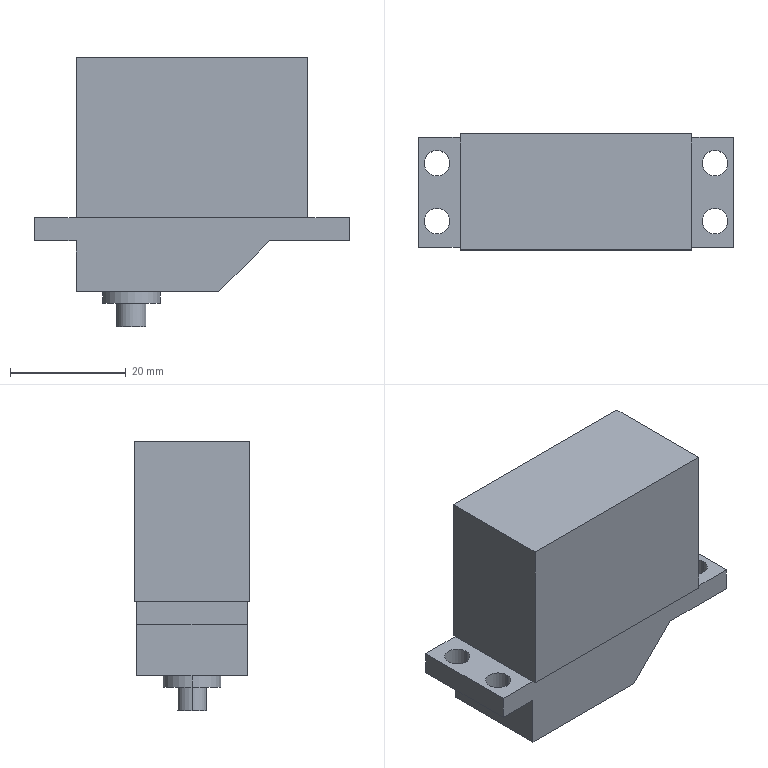Part | SolidWorks | features MirrorStock 1 | 1 solid | 32 faces | box 54.44 x 20 x 46.45 mm | volume 31100 mm3 | plane 20 | cylinder 12 | commonest cylinder face diameters 4.4 x8 5 x2 10 x2
STEP:
#1=CARTESIAN_POINT('',(-12.95,0.,-46.45));
#2=VERTEX_POINT('',#1);
#3=CARTESIAN_POINT('',(-7.95,0.,-46.45));
#4=VERTEX_POINT('',#3);
#5=CARTESIAN_POINT('',(-10.45,0.,-46.45));
#6=DIRECTION('',(0.,0.,1.));
#7=DIRECTION('',(1.,0.,0.));
#8=AXIS2_PLACEMENT_3D('',#5,#6,#7);
#9=CIRCLE('',#8,2.5);
#10=EDGE_CURVE('',#2,#4,#9,.T.);
#11=ORIENTED_EDGE('',*,*,#10,.T.);
#12=CARTESIAN_POINT('',(-7.95,0.,-42.45));
#13=VERTEX_POINT('',#12);
#14=CARTESIAN_POINT('',(-7.95,0.,-46.45));
#15=DIRECTION('',(0.,0.,1.));
#16=VECTOR('',#15,1000.);
#17=LINE('',#14,#16);
#18=EDGE_CURVE('',#4,#13,#17,.T.);
#19=ORIENTED_EDGE('',*,*,#18,.T.);
#20=CARTESIAN_POINT('',(-12.95,0.,-42.45));
#21=VERTEX_POINT('',#20);
#22=CARTESIAN_POINT('',(-10.45,0.,-42.45));
#23=DIRECTION('',(0.,0.,1.));
#24=DIRECTION('',(1.,0.,0.));
#25=AXIS2_PLACEMENT_3D('',#22,#23,#24);
#26=CIRCLE('',#25,2.5);
#27=EDGE_CURVE('',#21,#13,#26,.T.);
#28=ORIENTED_EDGE('',*,*,#27,.F.);
#29=CARTESIAN_POINT('',(-12.95,0.,-46.45));
#30=DIRECTION('',(0.,0.,1.));
#31=VECTOR('',#30,1000.);
#32=LINE('',#29,#31);
#33=EDGE_CURVE('',#2,#21,#32,.T.);
#34=ORIENTED_EDGE('',*,*,#33,.F.);
#35=EDGE_LOOP('',(#11,#19,#28,#34));
#36=FACE_OUTER_BOUND('',#35,.T.);
#37=CARTESIAN_POINT('',(-10.45,0.,-46.45));
#38=DIRECTION('',(0.,0.,1.));
#39=DIRECTION('',(-1.,0.,0.));
#40=AXIS2_PLACEMENT_3D('',#37,#38,#39);
#41=CYLINDRICAL_SURFACE('',#40,2.5);
#42=ADVANCED_FACE('',(#36),#41,.T.);
#43=CARTESIAN_POINT('',(-15.45,0.,-42.45));
#44=VERTEX_POINT('',#43);
#45=CARTESIAN_POINT('',(-5.45,0.,-42.45));
#46=VERTEX_POINT('',#45);
#47=CARTESIAN_POINT('',(-10.45,0.,-42.45));
#48=DIRECTION('',(0.,0.,1.));
#49=DIRECTION('',(1.,0.,0.));
#50=AXIS2_PLACEMENT_3D('',#47,#48,#49);
#51=CIRCLE('',#50,5.);
#52=EDGE_CURVE('',#44,#46,#51,.T.);
#53=ORIENTED_EDGE('',*,*,#52,.T.);
#54=CARTESIAN_POINT('',(-5.45,0.,-40.45));
#55=VERTEX_POINT('',#54);
#56=CARTESIAN_POINT('',(-5.45,0.,-42.45));
#57=DIRECTION('',(0.,0.,1.));
#58=VECTOR('',#57,1000.);
#59=LINE('',#56,#58);
#60=EDGE_CURVE('',#46,#55,#59,.T.);
#61=ORIENTED_EDGE('',*,*,#60,.T.);
#62=CARTESIAN_POINT('',(-15.45,0.,-40.45));
#63=VERTEX_POINT('',#62);
#64=CARTESIAN_POINT('',(-10.45,0.,-40.45));
#65=DIRECTION('',(0.,0.,1.));
#66=DIRECTION('',(1.,0.,0.));
#67=AXIS2_PLACEMENT_3D('',#64,#65,#66);
#68=CIRCLE('',#67,5.);
#69=EDGE_CURVE('',#63,#55,#68,.T.);
#70=ORIENTED_EDGE('',*,*,#69,.F.);
#71=CARTESIAN_POINT('',(-15.45,0.,-42.45));
#72=DIRECTION('',(0.,0.,1.));
#73=VECTOR('',#72,1000.);
#74=LINE('',#71,#73);
#75=EDGE_CURVE('',#44,#63,#74,.T.);
#76=ORIENTED_EDGE('',*,*,#75,.F.);
#77=EDGE_LOOP('',(#53,#61,#70,#76));
#78=FACE_OUTER_BOUND('',#77,.T.);
#79=CARTESIAN_POINT('',(-10.45,0.,-42.45));
#80=DIRECTION('',(0.,0.,1.));
#81=DIRECTION('',(-1.,0.,0.));
#82=AXIS2_PLACEMENT_3D('',#79,#80,#81);
#83=CYLINDRICAL_SURFACE('',#82,5.);
#84=ADVANCED_FACE('',(#78),#83,.T.);
#85=CARTESIAN_POINT('',(26.2,5.,-27.65));
#86=VERTEX_POINT('',#85);
#87=CARTESIAN_POINT('',(21.8,5.,-27.65));
#88=VERTEX_POINT('',#87);
#89=CARTESIAN_POINT('',(24.,5.,-27.65));
#90=DIRECTION('',(0.,0.,1.));
#91=DIRECTION('',(1.,0.,0.));
#92=AXIS2_PLACEMENT_3D('',#89,#90,#91);
#93=CIRCLE('',#92,2.2);
#94=EDGE_CURVE('',#86,#88,#93,.T.);
#95=ORIENTED_EDGE('',*,*,#94,.T.);
#96=CARTESIAN_POINT('',(21.8,5.,-31.65));
#97=VERTEX_POINT('',#96);
#98=CARTESIAN_POINT('',(21.8,5.,-27.65));
#99=DIRECTION('',(0.,0.,-1.));
#100=VECTOR('',#99,1000.);
#101=LINE('',#98,#100);
#102=EDGE_CURVE('',#88,#97,#101,.T.);
#103=ORIENTED_EDGE('',*,*,#102,.T.);
#104=CARTESIAN_POINT('',(26.2,5.,-31.65));
#105=VERTEX_POINT('',#104);
#106=CARTESIAN_POINT('',(24.,5.,-31.65));
#107=DIRECTION('',(0.,0.,1.));
#108=DIRECTION('',(1.,0.,0.));
#109=AXIS2_PLACEMENT_3D('',#106,#107,#108);
#110=CIRCLE('',#109,2.2);
#111=EDGE_CURVE('',#105,#97,#110,.T.);
#112=ORIENTED_EDGE('',*,*,#111,.F.);
#113=CARTESIAN_POINT('',(26.2,5.,-27.65));
#114=DIRECTION('',(0.,0.,-1.));
#115=VECTOR('',#114,1000.);
#116=LINE('',#113,#115);
#117=EDGE_CURVE('',#86,#105,#116,.T.);
#118=ORIENTED_EDGE('',*,*,#117,.F.);
#119=EDGE_LOOP('',(#95,#103,#112,#118));
#120=FACE_OUTER_BOUND('',#119,.T.);
#121=CARTESIAN_POINT('',(24.,5.,-27.65));
#122=DIRECTION('',(0.,0.,-1.));
#123=DIRECTION('',(1.,0.,0.));
#124=AXIS2_PLACEMENT_3D('',#121,#122,#123);
#125=CYLINDRICAL_SURFACE('',#124,2.2);
#126=ADVANCED_FACE('',(#120),#125,.F.);
#127=CARTESIAN_POINT('',(26.2,-5.,-27.65));
#128=VERTEX_POINT('',#127);
#129=CARTESIAN_POINT('',(21.8,-5.,-27.65));
#130=VERTEX_POINT('',#129);
#131=CARTESIAN_POINT('',(24.,-5.,-27.65));
#132=DIRECTION('',(0.,0.,1.));
#133=DIRECTION('',(1.,0.,0.));
#134=AXIS2_PLACEMENT_3D('',#131,#132,#133);
#135=CIRCLE('',#134,2.2);
#136=EDGE_CURVE('',#128,#130,#135,.T.);
#137=ORIENTED_EDGE('',*,*,#136,.T.);
#138=CARTESIAN_POINT('',(21.8,-5.,-31.65));
#139=VERTEX_POINT('',#138);
#140=CARTESIAN_POINT('',(21.8,-5.,-27.65));
#141=DIRECTION('',(0.,0.,-1.));
#142=VECTOR('',#141,1000.);
#143=LINE('',#140,#142);
#144=EDGE_CURVE('',#130,#139,#143,.T.);
#145=ORIENTED_EDGE('',*,*,#144,.T.);
#146=CARTESIAN_POINT('',(26.2,-5.,-31.65));
#147=VERTEX_POINT('',#146);
#148=CARTESIAN_POINT('',(24.,-5.,-31.65));
#149=DIRECTION('',(0.,0.,1.));
#150=DIRECTION('',(1.,0.,0.));
#151=AXIS2_PLACEMENT_3D('',#148,#149,#150);
#152=CIRCLE('',#151,2.2);
#153=EDGE_CURVE('',#147,#139,#152,.T.);
#154=ORIENTED_EDGE('',*,*,#153,.F.);
#155=CARTESIAN_POINT('',(26.2,-5.,-27.65));
#156=DIRECTION('',(0.,0.,-1.));
#157=VECTOR('',#156,1000.);
#158=LINE('',#155,#157);
#159=EDGE_CURVE('',#128,#147,#158,.T.);
#160=ORIENTED_EDGE('',*,*,#159,.F.);
#161=EDGE_LOOP('',(#137,#145,#154,#160));
#162=FACE_OUTER_BOUND('',#161,.T.);
#163=CARTESIAN_POINT('',(24.,-5.,-27.65));
#164=DIRECTION('',(0.,0.,-1.));
#165=DIRECTION('',(1.,0.,0.));
#166=AXIS2_PLACEMENT_3D('',#163,#164,#165);
#167=CYLINDRICAL_SURFACE('',#166,2.2);
#168=ADVANCED_FACE('',(#162),#167,.F.);
#169=CARTESIAN_POINT('',(-21.8,-5.,-27.65));
#170=VERTEX_POINT('',#169);
#171=CARTESIAN_POINT('',(-26.2,-5.,-27.65));
#172=VERTEX_POINT('',#171);
#173=CARTESIAN_POINT('',(-24.,-5.,-27.65));
#174=DIRECTION('',(0.,0.,1.));
#175=DIRECTION('',(1.,0.,0.));
#176=AXIS2_PLACEMENT_3D('',#173,#174,#175);
#177=CIRCLE('',#176,2.2);
#178=EDGE_CURVE('',#170,#172,#177,.T.);
#179=ORIENTED_EDGE('',*,*,#178,.T.);
#180=CARTESIAN_POINT('',(-26.2,-5.,-31.65));
#181=VERTEX_POINT('',#180);
#182=CARTESIAN_POINT('',(-26.2,-5.,-27.65));
#183=DIRECTION('',(0.,0.,-1.));
#184=VECTOR('',#183,1000.);
#185=LINE('',#182,#184);
#186=EDGE_CURVE('',#172,#181,#185,.T.);
#187=ORIENTED_EDGE('',*,*,#186,.T.);
#188=CARTESIAN_POINT('',(-21.8,-5.,-31.65));
#189=VERTEX_POINT('',#188);
#190=CARTESIAN_POINT('',(-24.,-5.,-31.65));
#191=DIRECTION('',(0.,0.,1.));
#192=DIRECTION('',(1.,0.,0.));
#193=AXIS2_PLACEMENT_3D('',#190,#191,#192);
#194=CIRCLE('',#193,2.2);
#195=EDGE_CURVE('',#189,#181,#194,.T.);
#196=ORIENTED_EDGE('',*,*,#195,.F.);
#197=CARTESIAN_POINT('',(-21.8,-5.,-27.65));
#198=DIRECTION('',(0.,0.,-1.));
#199=VECTOR('',#198,1000.);
#200=LINE('',#197,#199);
#201=EDGE_CURVE('',#170,#189,#200,.T.);
#202=ORIENTED_EDGE('',*,*,#201,.F.);
#203=EDGE_LOOP('',(#179,#187,#196,#202));
#204=FACE_OUTER_BOUND('',#203,.T.);
#205=CARTESIAN_POINT('',(-24.,-5.,-27.65));
#206=DIRECTION('',(0.,0.,-1.));
#207=DIRECTION('',(1.,0.,0.));
#208=AXIS2_PLACEMENT_3D('',#205,#206,#207);
#209=CYLINDRICAL_SURFACE('',#208,2.2);
#210=ADVANCED_FACE('',(#204),#209,.F.);
#211=CARTESIAN_POINT('',(-21.8,5.,-27.65));
#212=VERTEX_POINT('',#211);
#213=CARTESIAN_POINT('',(-26.2,5.,-27.65));
#214=VERTEX_POINT('',#213);
#215=CARTESIAN_POINT('',(-24.,5.,-27.65));
#216=DIRECTION('',(0.,0.,1.));
#217=DIRECTION('',(1.,0.,0.));
#218=AXIS2_PLACEMENT_3D('',#215,#216,#217);
#219=CIRCLE('',#218,2.2);
#220=EDGE_CURVE('',#212,#214,#219,.T.);
#221=ORIENTED_EDGE('',*,*,#220,.T.);
#222=CARTESIAN_POINT('',(-26.2,5.,-31.65));
#223=VERTEX_POINT('',#222);
#224=CARTESIAN_POINT('',(-26.2,5.,-27.65));
#225=DIRECTION('',(0.,0.,-1.));
#226=VECTOR('',#225,1000.);
#227=LINE('',#224,#226);
#228=EDGE_CURVE('',#214,#223,#227,.T.);
#229=ORIENTED_EDGE('',*,*,#228,.T.);
#230=CARTESIAN_POINT('',(-21.8,5.,-31.65));
#231=VERTEX_POINT('',#230);
#232=CARTESIAN_POINT('',(-24.,5.,-31.65));
#233=DIRECTION('',(0.,0.,1.));
#234=DIRECTION('',(1.,0.,0.));
#235=AXIS2_PLACEMENT_3D('',#232,#233,#234);
#236=CIRCLE('',#235,2.2);
#237=EDGE_CURVE('',#231,#223,#236,.T.);
#238=ORIENTED_EDGE('',*,*,#237,.F.);
#239=CARTESIAN_POINT('',(-21.8,5.,-27.65));
#240=DIRECTION('',(0.,0.,-1.));
#241=VECTOR('',#240,1000.);
#242=LINE('',#239,#241);
#243=EDGE_CURVE('',#212,#231,#242,.T.);
#244=ORIENTED_EDGE('',*,*,#243,.F.);
#245=EDGE_LOOP('',(#221,#229,#238,#244));
#246=FACE_OUTER_BOUND('',#245,.T.);
#247=CARTESIAN_POINT('',(-24.,5.,-27.65));
#248=DIRECTION('',(0.,0.,-1.));
#249=DIRECTION('',(1.,0.,0.));
#250=AXIS2_PLACEMENT_3D('',#247,#248,#249);
#251=CYLINDRICAL_SURFACE('',#250,2.2);
#252=ADVANCED_FACE('',(#246),#251,.F.);
#253=CARTESIAN_POINT('',(-20.,9.5,-31.65));
#254=VERTEX_POINT('',#253);
#255=CARTESIAN_POINT('',(-20.,-9.5,-31.65));
#256=VERTEX_POINT('',#255);
#257=CARTESIAN_POINT('',(-20.,-9.5,-31.65));
#258=DIRECTION('',(0.,-1.,0.));
#259=VECTOR('',#258,1000.);
#260=LINE('',#257,#259);
#261=EDGE_CURVE('',#254,#256,#260,.T.);
#262=ORIENTED_EDGE('',*,*,#261,.T.);
#263=CARTESIAN_POINT('',(-27.22,-9.5,-31.65));
#264=VERTEX_POINT('',#263);
#265=CARTESIAN_POINT('',(27.22,-9.5,-31.65));
#266=DIRECTION('',(1.,0.,0.));
#267=VECTOR('',#266,1000.);
#268=LINE('',#265,#267);
#269=EDGE_CURVE('',#264,#256,#268,.T.);
#270=ORIENTED_EDGE('',*,*,#269,.F.);
#271=CARTESIAN_POINT('',(-27.22,9.5,-31.65));
#272=VERTEX_POINT('',#271);
#273=CARTESIAN_POINT('',(-27.22,-9.5,-31.65));
#274=DIRECTION('',(0.,-1.,0.));
#275=VECTOR('',#274,1000.);
#276=LINE('',#273,#275);
#277=EDGE_CURVE('',#272,#264,#276,.T.);
#278=ORIENTED_EDGE('',*,*,#277,.F.);
#279=CARTESIAN_POINT('',(27.22,9.5,-31.65));
#280=DIRECTION('',(-1.,0.,0.));
#281=VECTOR('',#280,1000.);
#282=LINE('',#279,#281);
#283=EDGE_CURVE('',#254,#272,#282,.T.);
#284=ORIENTED_EDGE('',*,*,#283,.F.);
#285=EDGE_LOOP('',(#262,#270,#278,#284));
#286=FACE_OUTER_BOUND('',#285,.T.);
#287=ORIENTED_EDGE('',*,*,#237,.T.);
#288=CARTESIAN_POINT('',(-24.,5.,-31.65));
#289=DIRECTION('',(0.,0.,1.));
#290=DIRECTION('',(1.,0.,0.));
#291=AXIS2_PLACEMENT_3D('',#288,#289,#290);
#292=CIRCLE('',#291,2.2);
#293=EDGE_CURVE('',#223,#231,#292,.T.);
#294=ORIENTED_EDGE('',*,*,#293,.T.);
#295=EDGE_LOOP('',(#287,#294));
#296=FACE_BOUND('',#295,.T.);
#297=ORIENTED_EDGE('',*,*,#195,.T.);
#298=CARTESIAN_POINT('',(-24.,-5.,-31.65));
#299=DIRECTION('',(0.,0.,1.));
#300=DIRECTION('',(1.,0.,0.));
#301=AXIS2_PLACEMENT_3D('',#298,#299,#300);
#302=CIRCLE('',#301,2.2);
#303=EDGE_CURVE('',#181,#189,#302,.T.);
#304=ORIENTED_EDGE('',*,*,#303,.T.);
#305=EDGE_LOOP('',(#297,#304));
#306=FACE_BOUND('',#305,.T.);
#307=CARTESIAN_POINT('',(0.,0.,-31.65));
#308=DIRECTION('',(0.,0.,-1.));
#309=DIRECTION('',(1.,0.,0.));
#310=AXIS2_PLACEMENT_3D('',#307,#308,#309);
#311=PLANE('',#310);
#312=ADVANCED_FACE('',(#286,#296,#306),#311,.T.);
#313=CARTESIAN_POINT('',(20.,9.5,-27.65));
#314=VERTEX_POINT('',#313);
#315=CARTESIAN_POINT('',(-20.,9.5,-27.65));
#316=VERTEX_POINT('',#315);
#317=CARTESIAN_POINT('',(27.22,9.5,-27.65));
#318=DIRECTION('',(-1.,0.,0.));
#319=VECTOR('',#318,1000.);
#320=LINE('',#317,#319);
#321=EDGE_CURVE('',#314,#316,#320,.T.);
#322=ORIENTED_EDGE('',*,*,#321,.T.);
#323=CARTESIAN_POINT('',(-20.,10.,-27.65));
#324=VERTEX_POINT('',#323);
#325=CARTESIAN_POINT('',(-20.,-10.,-27.65));
#326=DIRECTION('',(0.,-1.,0.));
#327=VECTOR('',#326,1000.);
#328=LINE('',#325,#327);
#329=EDGE_CURVE('',#324,#316,#328,.T.);
#330=ORIENTED_EDGE('',*,*,#329,.F.);
#331=CARTESIAN_POINT('',(20.,10.,-27.65));
#332=VERTEX_POINT('',#331);
#333=CARTESIAN_POINT('',(20.,10.,-27.65));
#334=DIRECTION('',(-1.,0.,0.));
#335=VECTOR('',#334,1000.);
#336=LINE('',#333,#335);
#337=EDGE_CURVE('',#332,#324,#336,.T.);
#338=ORIENTED_EDGE('',*,*,#337,.F.);
#339=CARTESIAN_POINT('',(20.,-10.,-27.65));
#340=DIRECTION('',(0.,1.,0.));
#341=VECTOR('',#340,1000.);
#342=LINE('',#339,#341);
#343=EDGE_CURVE('',#314,#332,#342,.T.);
#344=ORIENTED_EDGE('',*,*,#343,.F.);
#345=EDGE_LOOP('',(#322,#330,#338,#344));
#346=FACE_OUTER_BOUND('',#345,.T.);
#347=CARTESIAN_POINT('',(0.,0.,-27.65));
#348=DIRECTION('',(0.,0.,-1.));
#349=DIRECTION('',(1.,0.,0.));
#350=AXIS2_PLACEMENT_3D('',#347,#348,#349);
#351=PLANE('',#350);
#352=ADVANCED_FACE('',(#346),#351,.T.);
#353=CARTESIAN_POINT('',(-20.,10.,0.));
#354=VERTEX_POINT('',#353);
#355=CARTESIAN_POINT('',(-20.,-10.,0.));
#356=VERTEX_POINT('',#355);
#357=CARTESIAN_POINT('',(-20.,-10.,0.));
#358=DIRECTION('',(0.,-1.,0.));
#359=VECTOR('',#358,1000.);
#360=LINE('',#357,#359);
#361=EDGE_CURVE('',#354,#356,#360,.T.);
#362=ORIENTED_EDGE('',*,*,#361,.F.);
#363=CARTESIAN_POINT('',(-20.,10.,-27.65));
#364=DIRECTION('',(0.,0.,1.));
#365=VECTOR('',#364,1000.);
#366=LINE('',#363,#365);
#367=EDGE_CURVE('',#324,#354,#366,.T.);
#368=ORIENTED_EDGE('',*,*,#367,.F.);
#369=ORIENTED_EDGE('',*,*,#329,.T.);
#370=CARTESIAN_POINT('',(-20.,-9.5,-27.65));
#371=VERTEX_POINT('',#370);
#372=CARTESIAN_POINT('',(-20.,-10.,-27.65));
#373=DIRECTION('',(0.,-1.,0.));
#374=VECTOR('',#373,1000.);
#375=LINE('',#372,#374);
#376=EDGE_CURVE('',#316,#371,#375,.T.);
#377=ORIENTED_EDGE('',*,*,#376,.T.);
#378=CARTESIAN_POINT('',(-20.,-10.,-27.65));
#379=VERTEX_POINT('',#378);
#380=CARTESIAN_POINT('',(-20.,-10.,-27.65));
#381=DIRECTION('',(0.,-1.,0.));
#382=VECTOR('',#381,1000.);
#383=LINE('',#380,#382);
#384=EDGE_CURVE('',#371,#379,#383,.T.);
#385=ORIENTED_EDGE('',*,*,#384,.T.);
#386=CARTESIAN_POINT('',(-20.,-10.,-27.65));
#387=DIRECTION('',(0.,0.,1.));
#388=VECTOR('',#387,1000.);
#389=LINE('',#386,#388);
#390=EDGE_CURVE('',#379,#356,#389,.T.);
#391=ORIENTED_EDGE('',*,*,#390,.T.);
#392=EDGE_LOOP('',(#362,#368,#369,#377,#385,#391));
#393=FACE_OUTER_BOUND('',#392,.T.);
#394=CARTESIAN_POINT('',(-20.,-10.,-27.65));
#395=DIRECTION('',(1.,0.,0.));
#396=DIRECTION('',(0.,0.,1.));
#397=AXIS2_PLACEMENT_3D('',#394,#395,#396);
#398=PLANE('',#397);
#399=ADVANCED_FACE('',(#393),#398,.F.);
#400=CARTESIAN_POINT('',(20.,-10.,0.));
#401=VERTEX_POINT('',#400);
#402=CARTESIAN_POINT('',(20.,-10.,0.));
#403=DIRECTION('',(1.,0.,0.));
#404=VECTOR('',#403,1000.);
#405=LINE('',#402,#404);
#406=EDGE_CURVE('',#356,#401,#405,.T.);
#407=ORIENTED_EDGE('',*,*,#406,.F.);
#408=ORIENTED_EDGE('',*,*,#390,.F.);
#409=CARTESIAN_POINT('',(20.,-10.,-27.65));
#410=VERTEX_POINT('',#409);
#411=CARTESIAN_POINT('',(20.,-10.,-27.65));
#412=DIRECTION('',(1.,0.,0.));
#413=VECTOR('',#412,1000.);
#414=LINE('',#411,#413);
#415=EDGE_CURVE('',#379,#410,#414,.T.);
#416=ORIENTED_EDGE('',*,*,#415,.T.);
#417=CARTESIAN_POINT('',(20.,-10.,-27.65));
#418=DIRECTION('',(0.,0.,1.));
#419=VECTOR('',#418,1000.);
#420=LINE('',#417,#419);
#421=EDGE_CURVE('',#410,#401,#420,.T.);
#422=ORIENTED_EDGE('',*,*,#421,.T.);
#423=EDGE_LOOP('',(#407,#408,#416,#422));
#424=FACE_OUTER_BOUND('',#423,.T.);
#425=CARTESIAN_POINT('',(20.,-10.,-27.65));
#426=DIRECTION('',(0.,1.,0.));
#427=DIRECTION('',(-1.,0.,0.));
#428=AXIS2_PLACEMENT_3D('',#425,#426,#427);
#429=PLANE('',#428);
#430=ADVANCED_FACE('',(#424),#429,.F.);
#431=CARTESIAN_POINT('',(20.,10.,0.));
#432=VERTEX_POINT('',#431);
#433=CARTESIAN_POINT('',(20.,-10.,0.));
#434=DIRECTION('',(0.,1.,0.));
#435=VECTOR('',#434,1000.);
#436=LINE('',#433,#435);
#437=EDGE_CURVE('',#401,#432,#436,.T.);
#438=ORIENTED_EDGE('',*,*,#437,.F.);
#439=ORIENTED_EDGE('',*,*,#421,.F.);
#440=CARTESIAN_POINT('',(20.,-9.5,-27.65));
#441=VERTEX_POINT('',#440);
#442=CARTESIAN_POINT('',(20.,-10.,-27.65));
#443=DIRECTION('',(0.,1.,0.));
#444=VECTOR('',#443,1000.);
#445=LINE('',#442,#444);
#446=EDGE_CURVE('',#410,#441,#445,.T.);
#447=ORIENTED_EDGE('',*,*,#446,.T.);
#448=CARTESIAN_POINT('',(20.,-10.,-27.65));
#449=DIRECTION('',(0.,1.,0.));
#450=VECTOR('',#449,1000.);
#451=LINE('',#448,#450);
#452=EDGE_CURVE('',#441,#314,#451,.T.);
#453=ORIENTED_EDGE('',*,*,#452,.T.);
#454=ORIENTED_EDGE('',*,*,#343,.T.);
#455=CARTESIAN_POINT('',(20.,10.,-27.65));
#456=DIRECTION('',(0.,0.,1.));
#457=VECTOR('',#456,1000.);
#458=LINE('',#455,#457);
#459=EDGE_CURVE('',#332,#432,#458,.T.);
#460=ORIENTED_EDGE('',*,*,#459,.T.);
#461=EDGE_LOOP('',(#438,#439,#447,#453,#454,#460));
#462=FACE_OUTER_BOUND('',#461,.T.);
#463=CARTESIAN_POINT('',(20.,-10.,-27.65));
#464=DIRECTION('',(-1.,0.,0.));
#465=DIRECTION('',(0.,0.,-1.));
#466=AXIS2_PLACEMENT_3D('',#463,#464,#465);
#467=PLANE('',#466);
#468=ADVANCED_FACE('',(#462),#467,.F.);
#469=CARTESIAN_POINT('',(20.,10.,0.));
#470=DIRECTION('',(-1.,0.,0.));
#471=VECTOR('',#470,1000.);
#472=LINE('',#469,#471);
#473=EDGE_CURVE('',#432,#354,#472,.T.);
#474=ORIENTED_EDGE('',*,*,#473,.F.);
#475=ORIENTED_EDGE('',*,*,#459,.F.);
#476=ORIENTED_EDGE('',*,*,#337,.T.);
#477=ORIENTED_EDGE('',*,*,#367,.T.);
#478=EDGE_LOOP('',(#474,#475,#476,#477));
#479=FACE_OUTER_BOUND('',#478,.T.);
#480=CARTESIAN_POINT('',(20.,10.,-27.65));
#481=DIRECTION('',(0.,-1.,0.));
#482=DIRECTION('',(1.,0.,0.));
#483=AXIS2_PLACEMENT_3D('',#480,#481,#482);
#484=PLANE('',#483);
#485=ADVANCED_FACE('',(#479),#484,.F.);
#486=CARTESIAN_POINT('',(27.22,-9.5,-27.65));
#487=DIRECTION('',(1.,0.,0.));
#488=VECTOR('',#487,1000.);
#489=LINE('',#486,#488);
#490=EDGE_CURVE('',#371,#441,#489,.T.);
#491=ORIENTED_EDGE('',*,*,#490,.T.);
#492=ORIENTED_EDGE('',*,*,#446,.F.);
#493=ORIENTED_EDGE('',*,*,#415,.F.);
#494=ORIENTED_EDGE('',*,*,#384,.F.);
#495=EDGE_LOOP('',(#491,#492,#493,#494));
#496=FACE_OUTER_BOUND('',#495,.T.);
#497=CARTESIAN_POINT('',(0.,0.,-27.65));
#498=DIRECTION('',(0.,0.,-1.));
#499=DIRECTION('',(1.,0.,0.));
#500=AXIS2_PLACEMENT_3D('',#497,#498,#499);
#501=PLANE('',#500);
#502=ADVANCED_FACE('',(#496),#501,.T.);
#503=ORIENTED_EDGE('',*,*,#361,.T.);
#504=ORIENTED_EDGE('',*,*,#406,.T.);
#505=ORIENTED_EDGE('',*,*,#437,.T.);
#506=ORIENTED_EDGE('',*,*,#473,.T.);
#507=EDGE_LOOP('',(#503,#504,#505,#506));
#508=FACE_OUTER_BOUND('',#507,.T.);
#509=CARTESIAN_POINT('',(0.,0.,0.));
#510=DIRECTION('',(0.,0.,-1.));
#511=DIRECTION('',(1.,0.,0.));
#512=AXIS2_PLACEMENT_3D('',#509,#510,#511);
#513=PLANE('',#512);
#514=ADVANCED_FACE('',(#508),#513,.F.);
#515=ORIENTED_EDGE('',*,*,#178,.F.);
#516=CARTESIAN_POINT('',(-24.,-5.,-27.65));
#517=DIRECTION('',(0.,0.,1.));
#518=DIRECTION('',(1.,0.,0.));
#519=AXIS2_PLACEMENT_3D('',#516,#517,#518);
#520=CIRCLE('',#519,2.2);
#521=EDGE_CURVE('',#172,#170,#520,.T.);
#522=ORIENTED_EDGE('',*,*,#521,.F.);
#523=EDGE_LOOP('',(#515,#522));
#524=FACE_BOUND('',#523,.T.);
#525=ORIENTED_EDGE('',*,*,#220,.F.);
#526=CARTESIAN_POINT('',(-24.,5.,-27.65));
#527=DIRECTION('',(0.,0.,1.));
#528=DIRECTION('',(1.,0.,0.));
#529=AXIS2_PLACEMENT_3D('',#526,#527,#528);
#530=CIRCLE('',#529,2.2);
#531=EDGE_CURVE('',#214,#212,#530,.T.);
#532=ORIENTED_EDGE('',*,*,#531,.F.);
#533=EDGE_LOOP('',(#525,#532));
#534=FACE_BOUND('',#533,.T.);
#535=CARTESIAN_POINT('',(-27.22,9.5,-27.65));
#536=VERTEX_POINT('',#535);
#537=CARTESIAN_POINT('',(27.22,9.5,-27.65));
#538=DIRECTION('',(-1.,0.,0.));
#539=VECTOR('',#538,1000.);
#540=LINE('',#537,#539);
#541=EDGE_CURVE('',#316,#536,#540,.T.);
#542=ORIENTED_EDGE('',*,*,#541,.T.);
#543=CARTESIAN_POINT('',(-27.22,-9.5,-27.65));
#544=VERTEX_POINT('',#543);
#545=CARTESIAN_POINT('',(-27.22,-9.5,-27.65));
#546=DIRECTION('',(0.,-1.,0.));
#547=VECTOR('',#546,1000.);
#548=LINE('',#545,#547);
#549=EDGE_CURVE('',#536,#544,#548,.T.);
#550=ORIENTED_EDGE('',*,*,#549,.T.);
#551=CARTESIAN_POINT('',(27.22,-9.5,-27.65));
#552=DIRECTION('',(1.,0.,0.));
#553=VECTOR('',#552,1000.);
#554=LINE('',#551,#553);
#555=EDGE_CURVE('',#544,#371,#554,.T.);
#556=ORIENTED_EDGE('',*,*,#555,.T.);
#557=ORIENTED_EDGE('',*,*,#376,.F.);
#558=EDGE_LOOP('',(#542,#550,#556,#557));
#559=FACE_OUTER_BOUND('',#558,.T.);
#560=CARTESIAN_POINT('',(0.,0.,-27.65));
#561=DIRECTION('',(0.,0.,-1.));
#562=DIRECTION('',(1.,0.,0.));
#563=AXIS2_PLACEMENT_3D('',#560,#561,#562);
#564=PLANE('',#563);
#565=ADVANCED_FACE('',(#524,#534,#559),#564,.F.);
#566=ORIENTED_EDGE('',*,*,#94,.F.);
#567=CARTESIAN_POINT('',(24.,5.,-27.65));
#568=DIRECTION('',(0.,0.,1.));
#569=DIRECTION('',(1.,0.,0.));
#570=AXIS2_PLACEMENT_3D('',#567,#568,#569);
#571=CIRCLE('',#570,2.2);
#572=EDGE_CURVE('',#88,#86,#571,.T.);
#573=ORIENTED_EDGE('',*,*,#572,.F.);
#574=EDGE_LOOP('',(#566,#573));
#575=FACE_BOUND('',#574,.T.);
#576=ORIENTED_EDGE('',*,*,#136,.F.);
#577=CARTESIAN_POINT('',(24.,-5.,-27.65));
#578=DIRECTION('',(0.,0.,1.));
#579=DIRECTION('',(1.,0.,0.));
#580=AXIS2_PLACEMENT_3D('',#577,#578,#579);
#581=CIRCLE('',#580,2.2);
#582=EDGE_CURVE('',#130,#128,#581,.T.);
#583=ORIENTED_EDGE('',*,*,#582,.F.);
#584=EDGE_LOOP('',(#576,#583));
#585=FACE_BOUND('',#584,.T.);
#586=CARTESIAN_POINT('',(27.22,-9.5,-27.65));
#587=VERTEX_POINT('',#586);
#588=CARTESIAN_POINT('',(27.22,-9.5,-27.65));
#589=DIRECTION('',(1.,0.,0.));
#590=VECTOR('',#589,1000.);
#591=LINE('',#588,#590);
#592=EDGE_CURVE('',#441,#587,#591,.T.);
#593=ORIENTED_EDGE('',*,*,#592,.T.);
#594=CARTESIAN_POINT('',(27.22,9.5,-27.65));
#595=VERTEX_POINT('',#594);
#596=CARTESIAN_POINT('',(27.22,-9.5,-27.65));
#597=DIRECTION('',(0.,1.,0.));
#598=VECTOR('',#597,1000.);
#599=LINE('',#596,#598);
#600=EDGE_CURVE('',#587,#595,#599,.T.);
#601=ORIENTED_EDGE('',*,*,#600,.T.);
#602=CARTESIAN_POINT('',(27.22,9.5,-27.65));
#603=DIRECTION('',(-1.,0.,0.));
#604=VECTOR('',#603,1000.);
#605=LINE('',#602,#604);
#606=EDGE_CURVE('',#595,#314,#605,.T.);
#607=ORIENTED_EDGE('',*,*,#606,.T.);
#608=ORIENTED_EDGE('',*,*,#452,.F.);
#609=EDGE_LOOP('',(#593,#601,#607,#608));
#610=FACE_OUTER_BOUND('',#609,.T.);
#611=CARTESIAN_POINT('',(0.,0.,-27.65));
#612=DIRECTION('',(0.,0.,-1.));
#613=DIRECTION('',(1.,0.,0.));
#614=AXIS2_PLACEMENT_3D('',#611,#612,#613);
#615=PLANE('',#614);
#616=ADVANCED_FACE('',(#575,#585,#610),#615,.F.);
#617=ORIENTED_EDGE('',*,*,#549,.F.);
#618=CARTESIAN_POINT('',(-27.22,9.5,-31.65));
#619=DIRECTION('',(0.,0.,1.));
#620=VECTOR('',#619,1000.);
#621=LINE('',#618,#620);
#622=EDGE_CURVE('',#272,#536,#621,.T.);
#623=ORIENTED_EDGE('',*,*,#622,.F.);
#624=ORIENTED_EDGE('',*,*,#277,.T.);
#625=CARTESIAN_POINT('',(-27.22,-9.5,-31.65));
#626=DIRECTION('',(0.,0.,1.));
#627=VECTOR('',#626,1000.);
#628=LINE('',#625,#627);
#629=EDGE_CURVE('',#264,#544,#628,.T.);
#630=ORIENTED_EDGE('',*,*,#629,.T.);
#631=EDGE_LOOP('',(#617,#623,#624,#630));
#632=FACE_OUTER_BOUND('',#631,.T.);
#633=CARTESIAN_POINT('',(-27.22,-9.5,-31.65));
#634=DIRECTION('',(1.,0.,0.));
#635=DIRECTION('',(0.,0.,1.));
#636=AXIS2_PLACEMENT_3D('',#633,#634,#635);
#637=PLANE('',#636);
#638=ADVANCED_FACE('',(#632),#637,.F.);
#639=CARTESIAN_POINT('',(13.407,-9.5,-31.65));
#640=VERTEX_POINT('',#639);
#641=CARTESIAN_POINT('',(27.22,-9.5,-31.65));
#642=VERTEX_POINT('',#641);
#643=CARTESIAN_POINT('',(27.22,-9.5,-31.65));
#644=DIRECTION('',(1.,0.,0.));
#645=VECTOR('',#644,1000.);
#646=LINE('',#643,#645);
#647=EDGE_CURVE('',#640,#642,#646,.T.);
#648=ORIENTED_EDGE('',*,*,#647,.T.);
#649=CARTESIAN_POINT('',(27.22,-9.5,-31.65));
#650=DIRECTION('',(0.,0.,1.));
#651=VECTOR('',#650,1000.);
#652=LINE('',#649,#651);
#653=EDGE_CURVE('',#642,#587,#652,.T.);
#654=ORIENTED_EDGE('',*,*,#653,.T.);
#655=ORIENTED_EDGE('',*,*,#592,.F.);
#656=ORIENTED_EDGE('',*,*,#490,.F.);
#657=ORIENTED_EDGE('',*,*,#555,.F.);
#658=ORIENTED_EDGE('',*,*,#629,.F.);
#659=ORIENTED_EDGE('',*,*,#269,.T.);
#660=CARTESIAN_POINT('',(-20.,-9.5,-40.45));
#661=VERTEX_POINT('',#660);
#662=CARTESIAN_POINT('',(-20.,-9.5,-120.38));
#663=DIRECTION('',(0.,0.,1.));
#664=VECTOR('',#663,1000.);
#665=LINE('',#662,#664);
#666=EDGE_CURVE('',#661,#256,#665,.T.);
#667=ORIENTED_EDGE('',*,*,#666,.F.);
#668=CARTESIAN_POINT('',(4.607,-9.5,-40.45));
#669=VERTEX_POINT('',#668);
#670=CARTESIAN_POINT('',(14.607,-9.5,-40.45));
#671=DIRECTION('',(1.,0.,0.));
#672=VECTOR('',#671,1000.);
#673=LINE('',#670,#672);
#674=EDGE_CURVE('',#661,#669,#673,.T.);
#675=ORIENTED_EDGE('',*,*,#674,.T.);
#676=CARTESIAN_POINT('',(4.607,-9.5,-40.45));
#677=DIRECTION('',(-0.7071,0.,-0.7071));
#678=VECTOR('',#677,1000.);
#679=LINE('',#676,#678);
#680=EDGE_CURVE('',#640,#669,#679,.T.);
#681=ORIENTED_EDGE('',*,*,#680,.F.);
#682=EDGE_LOOP('',(#648,#654,#655,#656,#657,#658,#659,#667,#675,#681));
#683=FACE_OUTER_BOUND('',#682,.T.);
#684=CARTESIAN_POINT('',(27.22,-9.5,-31.65));
#685=DIRECTION('',(0.,1.,0.));
#686=DIRECTION('',(-1.,0.,0.));
#687=AXIS2_PLACEMENT_3D('',#684,#685,#686);
#688=PLANE('',#687);
#689=ADVANCED_FACE('',(#683),#688,.F.);
#690=ORIENTED_EDGE('',*,*,#600,.F.);
#691=ORIENTED_EDGE('',*,*,#653,.F.);
#692=CARTESIAN_POINT('',(27.22,9.5,-31.65));
#693=VERTEX_POINT('',#692);
#694=CARTESIAN_POINT('',(27.22,-9.5,-31.65));
#695=DIRECTION('',(0.,1.,0.));
#696=VECTOR('',#695,1000.);
#697=LINE('',#694,#696);
#698=EDGE_CURVE('',#642,#693,#697,.T.);
#699=ORIENTED_EDGE('',*,*,#698,.T.);
#700=CARTESIAN_POINT('',(27.22,9.5,-31.65));
#701=DIRECTION('',(0.,0.,1.));
#702=VECTOR('',#701,1000.);
#703=LINE('',#700,#702);
#704=EDGE_CURVE('',#693,#595,#703,.T.);
#705=ORIENTED_EDGE('',*,*,#704,.T.);
#706=EDGE_LOOP('',(#690,#691,#699,#705));
#707=FACE_OUTER_BOUND('',#706,.T.);
#708=CARTESIAN_POINT('',(27.22,-9.5,-31.65));
#709=DIRECTION('',(-1.,0.,0.));
#710=DIRECTION('',(0.,0.,-1.));
#711=AXIS2_PLACEMENT_3D('',#708,#709,#710);
#712=PLANE('',#711);
#713=ADVANCED_FACE('',(#707),#712,.F.);
#714=CARTESIAN_POINT('',(4.607,9.5,-40.45));
#715=VERTEX_POINT('',#714);
#716=CARTESIAN_POINT('',(13.407,9.5,-31.65));
#717=VERTEX_POINT('',#716);
#718=CARTESIAN_POINT('',(4.607,9.5,-40.45));
#719=DIRECTION('',(0.7071,0.,0.7071));
#720=VECTOR('',#719,1000.);
#721=LINE('',#718,#720);
#722=EDGE_CURVE('',#715,#717,#721,.T.);
#723=ORIENTED_EDGE('',*,*,#722,.F.);
#724=CARTESIAN_POINT('',(-20.,9.5,-40.45));
#725=VERTEX_POINT('',#724);
#726=CARTESIAN_POINT('',(14.607,9.5,-40.45));
#727=DIRECTION('',(-1.,0.,0.));
#728=VECTOR('',#727,1000.);
#729=LINE('',#726,#728);
#730=EDGE_CURVE('',#715,#725,#729,.T.);
#731=ORIENTED_EDGE('',*,*,#730,.T.);
#732=CARTESIAN_POINT('',(-20.,9.5,-120.38));
#733=DIRECTION('',(0.,0.,1.));
#734=VECTOR('',#733,1000.);
#735=LINE('',#732,#734);
#736=EDGE_CURVE('',#725,#254,#735,.T.);
#737=ORIENTED_EDGE('',*,*,#736,.T.);
#738=ORIENTED_EDGE('',*,*,#283,.T.);
#739=ORIENTED_EDGE('',*,*,#622,.T.);
#740=ORIENTED_EDGE('',*,*,#541,.F.);
#741=ORIENTED_EDGE('',*,*,#321,.F.);
#742=ORIENTED_EDGE('',*,*,#606,.F.);
#743=ORIENTED_EDGE('',*,*,#704,.F.);
#744=CARTESIAN_POINT('',(27.22,9.5,-31.65));
#745=DIRECTION('',(-1.,0.,0.));
#746=VECTOR('',#745,1000.);
#747=LINE('',#744,#746);
#748=EDGE_CURVE('',#693,#717,#747,.T.);
#749=ORIENTED_EDGE('',*,*,#748,.T.);
#750=EDGE_LOOP('',(#723,#731,#737,#738,#739,#740,#741,#742,#743,#749));
#751=FACE_OUTER_BOUND('',#750,.T.);
#752=CARTESIAN_POINT('',(27.22,9.5,-31.65));
#753=DIRECTION('',(0.,-1.,0.));
#754=DIRECTION('',(1.,0.,0.));
#755=AXIS2_PLACEMENT_3D('',#752,#753,#754);
#756=PLANE('',#755);
#757=ADVANCED_FACE('',(#751),#756,.F.);
#758=ORIENTED_EDGE('',*,*,#748,.F.);
#759=ORIENTED_EDGE('',*,*,#698,.F.);
#760=ORIENTED_EDGE('',*,*,#647,.F.);
#761=CARTESIAN_POINT('',(13.407,0.,-31.65));
#762=DIRECTION('',(0.,-1.,0.));
#763=VECTOR('',#762,1000.);
#764=LINE('',#761,#763);
#765=EDGE_CURVE('',#717,#640,#764,.T.);
#766=ORIENTED_EDGE('',*,*,#765,.F.);
#767=EDGE_LOOP('',(#758,#759,#760,#766));
#768=FACE_OUTER_BOUND('',#767,.T.);
#769=ORIENTED_EDGE('',*,*,#111,.T.);
#770=CARTESIAN_POINT('',(24.,5.,-31.65));
#771=DIRECTION('',(0.,0.,1.));
#772=DIRECTION('',(1.,0.,0.));
#773=AXIS2_PLACEMENT_3D('',#770,#771,#772);
#774=CIRCLE('',#773,2.2);
#775=EDGE_CURVE('',#97,#105,#774,.T.);
#776=ORIENTED_EDGE('',*,*,#775,.T.);
#777=EDGE_LOOP('',(#769,#776));
#778=FACE_BOUND('',#777,.T.);
#779=ORIENTED_EDGE('',*,*,#153,.T.);
#780=CARTESIAN_POINT('',(24.,-5.,-31.65));
#781=DIRECTION('',(0.,0.,1.));
#782=DIRECTION('',(1.,0.,0.));
#783=AXIS2_PLACEMENT_3D('',#780,#781,#782);
#784=CIRCLE('',#783,2.2);
#785=EDGE_CURVE('',#139,#147,#784,.T.);
#786=ORIENTED_EDGE('',*,*,#785,.T.);
#787=EDGE_LOOP('',(#779,#786));
#788=FACE_BOUND('',#787,.T.);
#789=CARTESIAN_POINT('',(0.,0.,-31.65));
#790=DIRECTION('',(0.,0.,-1.));
#791=DIRECTION('',(1.,0.,0.));
#792=AXIS2_PLACEMENT_3D('',#789,#790,#791);
#793=PLANE('',#792);
#794=ADVANCED_FACE('',(#768,#778,#788),#793,.T.);
#795=ORIENTED_EDGE('',*,*,#228,.F.);
#796=ORIENTED_EDGE('',*,*,#531,.T.);
#797=ORIENTED_EDGE('',*,*,#243,.T.);
#798=ORIENTED_EDGE('',*,*,#293,.F.);
#799=EDGE_LOOP('',(#795,#796,#797,#798));
#800=FACE_OUTER_BOUND('',#799,.T.);
#801=CARTESIAN_POINT('',(-24.,5.,-27.65));
#802=DIRECTION('',(0.,0.,-1.));
#803=DIRECTION('',(1.,0.,0.));
#804=AXIS2_PLACEMENT_3D('',#801,#802,#803);
#805=CYLINDRICAL_SURFACE('',#804,2.2);
#806=ADVANCED_FACE('',(#800),#805,.F.);
#807=ORIENTED_EDGE('',*,*,#186,.F.);
#808=ORIENTED_EDGE('',*,*,#521,.T.);
#809=ORIENTED_EDGE('',*,*,#201,.T.);
#810=ORIENTED_EDGE('',*,*,#303,.F.);
#811=EDGE_LOOP('',(#807,#808,#809,#810));
#812=FACE_OUTER_BOUND('',#811,.T.);
#813=CARTESIAN_POINT('',(-24.,-5.,-27.65));
#814=DIRECTION('',(0.,0.,-1.));
#815=DIRECTION('',(1.,0.,0.));
#816=AXIS2_PLACEMENT_3D('',#813,#814,#815);
#817=CYLINDRICAL_SURFACE('',#816,2.2);
#818=ADVANCED_FACE('',(#812),#817,.F.);
#819=ORIENTED_EDGE('',*,*,#144,.F.);
#820=ORIENTED_EDGE('',*,*,#582,.T.);
#821=ORIENTED_EDGE('',*,*,#159,.T.);
#822=ORIENTED_EDGE('',*,*,#785,.F.);
#823=EDGE_LOOP('',(#819,#820,#821,#822));
#824=FACE_OUTER_BOUND('',#823,.T.);
#825=CARTESIAN_POINT('',(24.,-5.,-27.65));
#826=DIRECTION('',(0.,0.,-1.));
#827=DIRECTION('',(1.,0.,0.));
#828=AXIS2_PLACEMENT_3D('',#825,#826,#827);
#829=CYLINDRICAL_SURFACE('',#828,2.2);
#830=ADVANCED_FACE('',(#824),#829,.F.);
#831=ORIENTED_EDGE('',*,*,#102,.F.);
#832=ORIENTED_EDGE('',*,*,#572,.T.);
#833=ORIENTED_EDGE('',*,*,#117,.T.);
#834=ORIENTED_EDGE('',*,*,#775,.F.);
#835=EDGE_LOOP('',(#831,#832,#833,#834));
#836=FACE_OUTER_BOUND('',#835,.T.);
#837=CARTESIAN_POINT('',(24.,5.,-27.65));
#838=DIRECTION('',(0.,0.,-1.));
#839=DIRECTION('',(1.,0.,0.));
#840=AXIS2_PLACEMENT_3D('',#837,#838,#839);
#841=CYLINDRICAL_SURFACE('',#840,2.2);
#842=ADVANCED_FACE('',(#836),#841,.F.);
#843=CARTESIAN_POINT('',(-20.,-9.5,-40.45));
#844=DIRECTION('',(0.,-1.,0.));
#845=VECTOR('',#844,1000.);
#846=LINE('',#843,#845);
#847=EDGE_CURVE('',#725,#661,#846,.T.);
#848=ORIENTED_EDGE('',*,*,#847,.T.);
#849=ORIENTED_EDGE('',*,*,#666,.T.);
#850=ORIENTED_EDGE('',*,*,#261,.F.);
#851=ORIENTED_EDGE('',*,*,#736,.F.);
#852=EDGE_LOOP('',(#848,#849,#850,#851));
#853=FACE_OUTER_BOUND('',#852,.T.);
#854=CARTESIAN_POINT('',(-20.,-9.5,-120.38));
#855=DIRECTION('',(1.,0.,0.));
#856=DIRECTION('',(0.,0.,1.));
#857=AXIS2_PLACEMENT_3D('',#854,#855,#856);
#858=PLANE('',#857);
#859=ADVANCED_FACE('',(#853),#858,.F.);
#860=ORIENTED_EDGE('',*,*,#69,.T.);
#861=CARTESIAN_POINT('',(-10.45,0.,-40.45));
#862=DIRECTION('',(0.,0.,1.));
#863=DIRECTION('',(1.,0.,0.));
#864=AXIS2_PLACEMENT_3D('',#861,#862,#863);
#865=CIRCLE('',#864,5.);
#866=EDGE_CURVE('',#55,#63,#865,.T.);
#867=ORIENTED_EDGE('',*,*,#866,.T.);
#868=EDGE_LOOP('',(#860,#867));
#869=FACE_BOUND('',#868,.T.);
#870=ORIENTED_EDGE('',*,*,#674,.F.);
#871=ORIENTED_EDGE('',*,*,#847,.F.);
#872=ORIENTED_EDGE('',*,*,#730,.F.);
#873=CARTESIAN_POINT('',(4.607,9.5,-40.45));
#874=DIRECTION('',(0.,1.,0.));
#875=VECTOR('',#874,1000.);
#876=LINE('',#873,#875);
#877=EDGE_CURVE('',#669,#715,#876,.T.);
#878=ORIENTED_EDGE('',*,*,#877,.F.);
#879=EDGE_LOOP('',(#870,#871,#872,#878));
#880=FACE_OUTER_BOUND('',#879,.T.);
#881=CARTESIAN_POINT('',(0.,0.,-40.45));
#882=DIRECTION('',(0.,0.,-1.));
#883=DIRECTION('',(1.,0.,0.));
#884=AXIS2_PLACEMENT_3D('',#881,#882,#883);
#885=PLANE('',#884);
#886=ADVANCED_FACE('',(#869,#880),#885,.T.);
#887=ORIENTED_EDGE('',*,*,#680,.T.);
#888=ORIENTED_EDGE('',*,*,#877,.T.);
#889=ORIENTED_EDGE('',*,*,#722,.T.);
#890=ORIENTED_EDGE('',*,*,#765,.T.);
#891=EDGE_LOOP('',(#887,#888,#889,#890));
#892=FACE_OUTER_BOUND('',#891,.T.);
#893=CARTESIAN_POINT('',(4.607,0.,-40.45));
#894=DIRECTION('',(0.7071,0.,-0.7071));
#895=DIRECTION('',(0.,-1.,0.));
#896=AXIS2_PLACEMENT_3D('',#893,#894,#895);
#897=PLANE('',#896);
#898=ADVANCED_FACE('',(#892),#897,.T.);
#899=ORIENTED_EDGE('',*,*,#60,.F.);
#900=CARTESIAN_POINT('',(-10.45,0.,-42.45));
#901=DIRECTION('',(0.,0.,1.));
#902=DIRECTION('',(1.,0.,0.));
#903=AXIS2_PLACEMENT_3D('',#900,#901,#902);
#904=CIRCLE('',#903,5.);
#905=EDGE_CURVE('',#46,#44,#904,.T.);
#906=ORIENTED_EDGE('',*,*,#905,.T.);
#907=ORIENTED_EDGE('',*,*,#75,.T.);
#908=ORIENTED_EDGE('',*,*,#866,.F.);
#909=EDGE_LOOP('',(#899,#906,#907,#908));
#910=FACE_OUTER_BOUND('',#909,.T.);
#911=CARTESIAN_POINT('',(-10.45,0.,-42.45));
#912=DIRECTION('',(0.,0.,1.));
#913=DIRECTION('',(-1.,0.,0.));
#914=AXIS2_PLACEMENT_3D('',#911,#912,#913);
#915=CYLINDRICAL_SURFACE('',#914,5.);
#916=ADVANCED_FACE('',(#910),#915,.T.);
#917=ORIENTED_EDGE('',*,*,#27,.T.);
#918=CARTESIAN_POINT('',(-10.45,0.,-42.45));
#919=DIRECTION('',(0.,0.,1.));
#920=DIRECTION('',(1.,0.,0.));
#921=AXIS2_PLACEMENT_3D('',#918,#919,#920);
#922=CIRCLE('',#921,2.5);
#923=EDGE_CURVE('',#13,#21,#922,.T.);
#924=ORIENTED_EDGE('',*,*,#923,.T.);
#925=EDGE_LOOP('',(#917,#924));
#926=FACE_BOUND('',#925,.T.);
#927=ORIENTED_EDGE('',*,*,#52,.F.);
#928=ORIENTED_EDGE('',*,*,#905,.F.);
#929=EDGE_LOOP('',(#927,#928));
#930=FACE_OUTER_BOUND('',#929,.T.);
#931=CARTESIAN_POINT('',(-10.45,0.,-42.45));
#932=DIRECTION('',(0.,0.,-1.));
#933=DIRECTION('',(1.,0.,0.));
#934=AXIS2_PLACEMENT_3D('',#931,#932,#933);
#935=PLANE('',#934);
#936=ADVANCED_FACE('',(#926,#930),#935,.T.);
#937=ORIENTED_EDGE('',*,*,#18,.F.);
#938=CARTESIAN_POINT('',(-10.45,0.,-46.45));
#939=DIRECTION('',(0.,0.,1.));
#940=DIRECTION('',(1.,0.,0.));
#941=AXIS2_PLACEMENT_3D('',#938,#939,#940);
#942=CIRCLE('',#941,2.5);
#943=EDGE_CURVE('',#4,#2,#942,.T.);
#944=ORIENTED_EDGE('',*,*,#943,.T.);
#945=ORIENTED_EDGE('',*,*,#33,.T.);
#946=ORIENTED_EDGE('',*,*,#923,.F.);
#947=EDGE_LOOP('',(#937,#944,#945,#946));
#948=FACE_OUTER_BOUND('',#947,.T.);
#949=CARTESIAN_POINT('',(-10.45,0.,-46.45));
#950=DIRECTION('',(0.,0.,1.));
#951=DIRECTION('',(-1.,0.,0.));
#952=AXIS2_PLACEMENT_3D('',#949,#950,#951);
#953=CYLINDRICAL_SURFACE('',#952,2.5);
#954=ADVANCED_FACE('',(#948),#953,.T.);
#955=ORIENTED_EDGE('',*,*,#10,.F.);
#956=ORIENTED_EDGE('',*,*,#943,.F.);
#957=EDGE_LOOP('',(#955,#956));
#958=FACE_OUTER_BOUND('',#957,.T.);
#959=CARTESIAN_POINT('',(-10.45,0.,-46.45));
#960=DIRECTION('',(0.,0.,-1.));
#961=DIRECTION('',(1.,0.,0.));
#962=AXIS2_PLACEMENT_3D('',#959,#960,#961);
#963=PLANE('',#962);
#964=ADVANCED_FACE('',(#958),#963,.T.);
#965=CLOSED_SHELL('',(#42,#84,#126,#168,#210,#252,#312,#352,#399,#430,#468,#485,#502,#514,#565,#616,#638,#689,#713,#757,#794,#806,#818,#830,#842,#859,#886,#898,#916,#936,#954,#964));
#966=MANIFOLD_SOLID_BREP('',#965);
#967=CARTESIAN_POINT('',(0.,0.,0.));
#968=DIRECTION('',(0.,0.,1.));
#969=DIRECTION('',(1.,0.,0.));
#970=AXIS2_PLACEMENT_3D('',#967,#968,#969);
#971=(LENGTH_UNIT()NAMED_UNIT(*)SI_UNIT(.MILLI.,.METRE.));
#972=UNCERTAINTY_MEASURE_WITH_UNIT(LENGTH_MEASURE(0.00001),#971,'','');
#973=(NAMED_UNIT(*)PLANE_ANGLE_UNIT()SI_UNIT($,.RADIAN.));
#974=(NAMED_UNIT(*)SI_UNIT($,.STERADIAN.)SOLID_ANGLE_UNIT());
#975=(GEOMETRIC_REPRESENTATION_CONTEXT(3)GLOBAL_UNCERTAINTY_ASSIGNED_CONTEXT((#972))GLOBAL_UNIT_ASSIGNED_CONTEXT((#971,#973,#974))REPRESENTATION_CONTEXT('',''));
#976=ADVANCED_BREP_SHAPE_REPRESENTATION('',(#966,#970),#975);